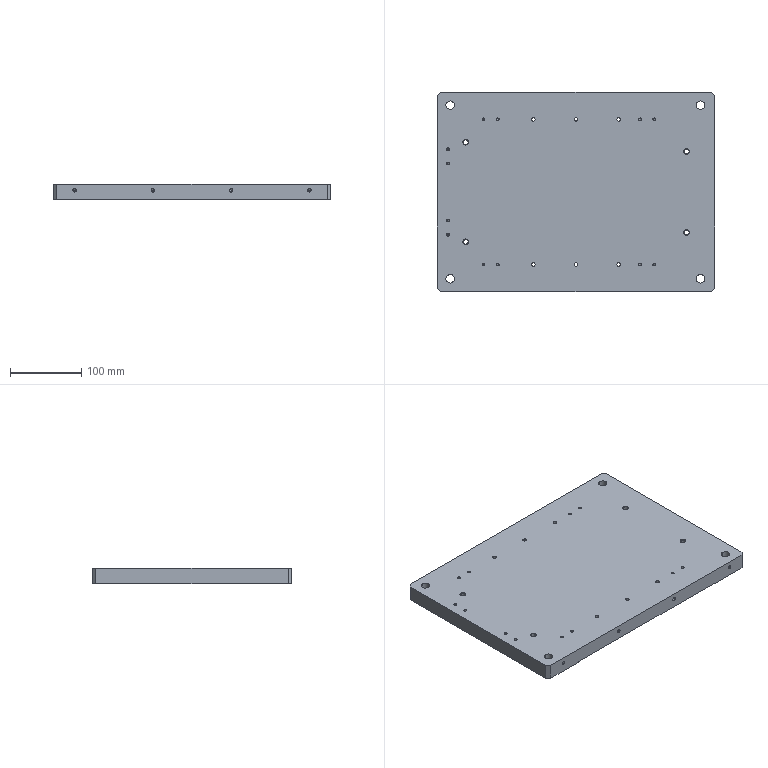Part | 1 solid | 170 faces | box 390 x 280 x 22 mm | volume 2307603 mm3 | cone 88 | cylinder 68 | plane 14 | commonest cylinder face diameters 3.3 x24 4.2 x16 5 x12 6.8 x8 12 x8